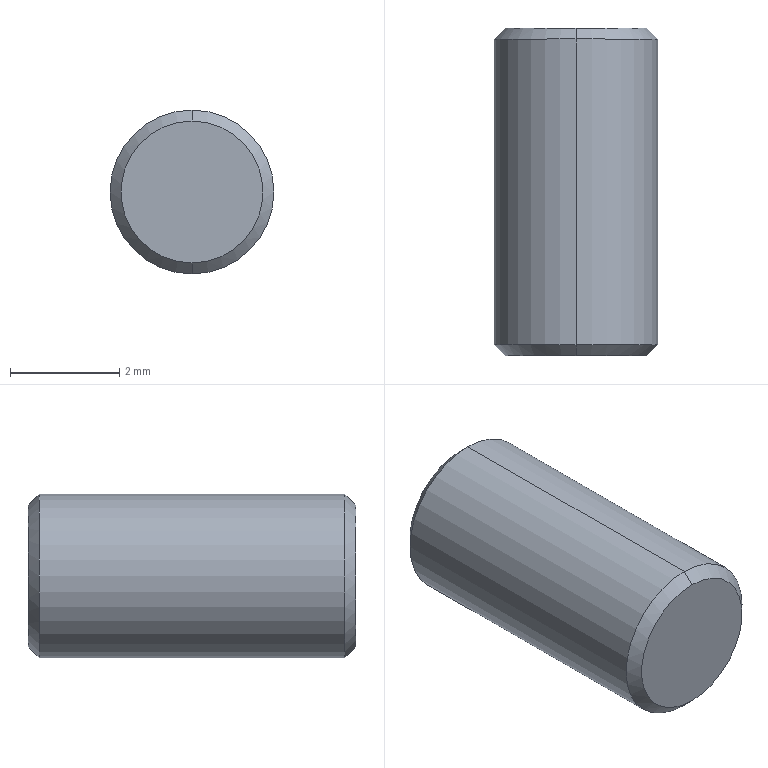Part | SolidWorks | features Chamfer 1, Extrusion 1 | 1 solid | 8 faces | box 3 x 6 x 3 mm | volume 42.051 mm3 | cone 4 | cylinder 2 | plane 2 | commonest cylinder face diameters 3 x2
STEP:
#1=CARTESIAN_POINT('',(0.,6.,1.3));
#2=VERTEX_POINT('',#1);
#3=CARTESIAN_POINT('',(0.,6.,-1.3));
#4=VERTEX_POINT('',#3);
#5=CARTESIAN_POINT('',(0.,6.,0.));
#6=DIRECTION('',(0.,1.,0.));
#7=DIRECTION('',(0.,0.,1.));
#8=AXIS2_PLACEMENT_3D('',#5,#6,#7);
#9=CIRCLE('',#8,1.3);
#10=EDGE_CURVE('',#2,#4,#9,.T.);
#11=ORIENTED_EDGE('',*,*,#10,.F.);
#12=CARTESIAN_POINT('',(0.,5.8,1.5));
#13=VERTEX_POINT('',#12);
#14=CARTESIAN_POINT('',(0.,6.,1.3));
#15=DIRECTION('',(0.,-0.7071,0.7071));
#16=VECTOR('',#15,1000.);
#17=LINE('',#14,#16);
#18=EDGE_CURVE('',#2,#13,#17,.T.);
#19=ORIENTED_EDGE('',*,*,#18,.T.);
#20=CARTESIAN_POINT('',(0.,5.8,-1.5));
#21=VERTEX_POINT('',#20);
#22=CARTESIAN_POINT('',(0.,5.8,0.));
#23=DIRECTION('',(0.,-1.,0.));
#24=DIRECTION('',(0.,0.,1.));
#25=AXIS2_PLACEMENT_3D('',#22,#23,#24);
#26=CIRCLE('',#25,1.5);
#27=EDGE_CURVE('',#21,#13,#26,.T.);
#28=ORIENTED_EDGE('',*,*,#27,.F.);
#29=CARTESIAN_POINT('',(0.,6.,-1.3));
#30=DIRECTION('',(0.,-0.7071,-0.7071));
#31=VECTOR('',#30,1000.);
#32=LINE('',#29,#31);
#33=EDGE_CURVE('',#4,#21,#32,.T.);
#34=ORIENTED_EDGE('',*,*,#33,.F.);
#35=EDGE_LOOP('',(#11,#19,#28,#34));
#36=FACE_OUTER_BOUND('',#35,.T.);
#37=CARTESIAN_POINT('',(0.,6.,0.));
#38=DIRECTION('',(0.,-1.,0.));
#39=DIRECTION('',(0.,0.,-1.));
#40=AXIS2_PLACEMENT_3D('',#37,#38,#39);
#41=CONICAL_SURFACE('',#40,1.3,0.7854);
#42=ADVANCED_FACE('',(#36),#41,.T.);
#43=CARTESIAN_POINT('',(0.,0.,-1.3));
#44=VERTEX_POINT('',#43);
#45=CARTESIAN_POINT('',(0.,0.,1.3));
#46=VERTEX_POINT('',#45);
#47=CARTESIAN_POINT('',(0.,0.,0.));
#48=DIRECTION('',(0.,-1.,0.));
#49=DIRECTION('',(0.,0.,1.));
#50=AXIS2_PLACEMENT_3D('',#47,#48,#49);
#51=CIRCLE('',#50,1.3);
#52=EDGE_CURVE('',#44,#46,#51,.T.);
#53=ORIENTED_EDGE('',*,*,#52,.F.);
#54=CARTESIAN_POINT('',(0.,0.2,-1.5));
#55=VERTEX_POINT('',#54);
#56=CARTESIAN_POINT('',(0.,0.2,-1.5));
#57=DIRECTION('',(0.,0.7071,-0.7071));
#58=VECTOR('',#57,1000.);
#59=LINE('',#56,#58);
#60=EDGE_CURVE('',#44,#55,#59,.T.);
#61=ORIENTED_EDGE('',*,*,#60,.T.);
#62=CARTESIAN_POINT('',(0.,0.2,1.5));
#63=VERTEX_POINT('',#62);
#64=CARTESIAN_POINT('',(0.,0.2,0.));
#65=DIRECTION('',(0.,1.,0.));
#66=DIRECTION('',(0.,0.,1.));
#67=AXIS2_PLACEMENT_3D('',#64,#65,#66);
#68=CIRCLE('',#67,1.5);
#69=EDGE_CURVE('',#63,#55,#68,.T.);
#70=ORIENTED_EDGE('',*,*,#69,.F.);
#71=CARTESIAN_POINT('',(0.,0.2,1.5));
#72=DIRECTION('',(0.,0.7071,0.7071));
#73=VECTOR('',#72,1000.);
#74=LINE('',#71,#73);
#75=EDGE_CURVE('',#46,#63,#74,.T.);
#76=ORIENTED_EDGE('',*,*,#75,.F.);
#77=EDGE_LOOP('',(#53,#61,#70,#76));
#78=FACE_OUTER_BOUND('',#77,.T.);
#79=CARTESIAN_POINT('',(0.,0.2,0.));
#80=DIRECTION('',(0.,1.,0.));
#81=DIRECTION('',(0.,0.,1.));
#82=AXIS2_PLACEMENT_3D('',#79,#80,#81);
#83=CONICAL_SURFACE('',#82,1.5,0.7854);
#84=ADVANCED_FACE('',(#78),#83,.T.);
#85=ORIENTED_EDGE('',*,*,#27,.T.);
#86=CARTESIAN_POINT('',(0.,6.,1.5));
#87=DIRECTION('',(0.,-1.,0.));
#88=VECTOR('',#87,1000.);
#89=LINE('',#86,#88);
#90=EDGE_CURVE('',#13,#63,#89,.T.);
#91=ORIENTED_EDGE('',*,*,#90,.T.);
#92=ORIENTED_EDGE('',*,*,#69,.T.);
#93=CARTESIAN_POINT('',(0.,6.,-1.5));
#94=DIRECTION('',(0.,-1.,0.));
#95=VECTOR('',#94,1000.);
#96=LINE('',#93,#95);
#97=EDGE_CURVE('',#21,#55,#96,.T.);
#98=ORIENTED_EDGE('',*,*,#97,.F.);
#99=EDGE_LOOP('',(#85,#91,#92,#98));
#100=FACE_OUTER_BOUND('',#99,.T.);
#101=CARTESIAN_POINT('',(0.,6.,0.));
#102=DIRECTION('',(0.,-1.,0.));
#103=DIRECTION('',(0.,0.,-1.));
#104=AXIS2_PLACEMENT_3D('',#101,#102,#103);
#105=CYLINDRICAL_SURFACE('',#104,1.5);
#106=ADVANCED_FACE('',(#100),#105,.T.);
#107=ORIENTED_EDGE('',*,*,#90,.F.);
#108=CARTESIAN_POINT('',(0.,5.8,0.));
#109=DIRECTION('',(0.,-1.,0.));
#110=DIRECTION('',(0.,0.,1.));
#111=AXIS2_PLACEMENT_3D('',#108,#109,#110);
#112=CIRCLE('',#111,1.5);
#113=EDGE_CURVE('',#13,#21,#112,.T.);
#114=ORIENTED_EDGE('',*,*,#113,.T.);
#115=ORIENTED_EDGE('',*,*,#97,.T.);
#116=CARTESIAN_POINT('',(0.,0.2,0.));
#117=DIRECTION('',(0.,1.,0.));
#118=DIRECTION('',(0.,0.,1.));
#119=AXIS2_PLACEMENT_3D('',#116,#117,#118);
#120=CIRCLE('',#119,1.5);
#121=EDGE_CURVE('',#55,#63,#120,.T.);
#122=ORIENTED_EDGE('',*,*,#121,.T.);
#123=EDGE_LOOP('',(#107,#114,#115,#122));
#124=FACE_OUTER_BOUND('',#123,.T.);
#125=CARTESIAN_POINT('',(0.,6.,0.));
#126=DIRECTION('',(0.,-1.,0.));
#127=DIRECTION('',(0.,0.,-1.));
#128=AXIS2_PLACEMENT_3D('',#125,#126,#127);
#129=CYLINDRICAL_SURFACE('',#128,1.5);
#130=ADVANCED_FACE('',(#124),#129,.T.);
#131=CARTESIAN_POINT('',(0.,6.,0.));
#132=DIRECTION('',(0.,1.,0.));
#133=DIRECTION('',(0.,0.,1.));
#134=AXIS2_PLACEMENT_3D('',#131,#132,#133);
#135=CIRCLE('',#134,1.3);
#136=EDGE_CURVE('',#4,#2,#135,.T.);
#137=ORIENTED_EDGE('',*,*,#136,.T.);
#138=ORIENTED_EDGE('',*,*,#10,.T.);
#139=EDGE_LOOP('',(#137,#138));
#140=FACE_OUTER_BOUND('',#139,.T.);
#141=CARTESIAN_POINT('',(0.,6.,0.));
#142=DIRECTION('',(0.,1.,0.));
#143=DIRECTION('',(0.,0.,1.));
#144=AXIS2_PLACEMENT_3D('',#141,#142,#143);
#145=PLANE('',#144);
#146=ADVANCED_FACE('',(#140),#145,.T.);
#147=CARTESIAN_POINT('',(0.,0.,0.));
#148=DIRECTION('',(0.,-1.,0.));
#149=DIRECTION('',(0.,0.,1.));
#150=AXIS2_PLACEMENT_3D('',#147,#148,#149);
#151=CIRCLE('',#150,1.3);
#152=EDGE_CURVE('',#46,#44,#151,.T.);
#153=ORIENTED_EDGE('',*,*,#152,.T.);
#154=ORIENTED_EDGE('',*,*,#52,.T.);
#155=EDGE_LOOP('',(#153,#154));
#156=FACE_OUTER_BOUND('',#155,.T.);
#157=CARTESIAN_POINT('',(0.,0.,0.));
#158=DIRECTION('',(0.,1.,0.));
#159=DIRECTION('',(0.,0.,1.));
#160=AXIS2_PLACEMENT_3D('',#157,#158,#159);
#161=PLANE('',#160);
#162=ADVANCED_FACE('',(#156),#161,.F.);
#163=ORIENTED_EDGE('',*,*,#60,.F.);
#164=ORIENTED_EDGE('',*,*,#152,.F.);
#165=ORIENTED_EDGE('',*,*,#75,.T.);
#166=ORIENTED_EDGE('',*,*,#121,.F.);
#167=EDGE_LOOP('',(#163,#164,#165,#166));
#168=FACE_OUTER_BOUND('',#167,.T.);
#169=CARTESIAN_POINT('',(0.,0.2,0.));
#170=DIRECTION('',(0.,1.,0.));
#171=DIRECTION('',(0.,0.,1.));
#172=AXIS2_PLACEMENT_3D('',#169,#170,#171);
#173=CONICAL_SURFACE('',#172,1.5,0.7854);
#174=ADVANCED_FACE('',(#168),#173,.T.);
#175=ORIENTED_EDGE('',*,*,#18,.F.);
#176=ORIENTED_EDGE('',*,*,#136,.F.);
#177=ORIENTED_EDGE('',*,*,#33,.T.);
#178=ORIENTED_EDGE('',*,*,#113,.F.);
#179=EDGE_LOOP('',(#175,#176,#177,#178));
#180=FACE_OUTER_BOUND('',#179,.T.);
#181=CARTESIAN_POINT('',(0.,6.,0.));
#182=DIRECTION('',(0.,-1.,0.));
#183=DIRECTION('',(0.,0.,-1.));
#184=AXIS2_PLACEMENT_3D('',#181,#182,#183);
#185=CONICAL_SURFACE('',#184,1.3,0.7854);
#186=ADVANCED_FACE('',(#180),#185,.T.);
#187=CLOSED_SHELL('',(#42,#84,#106,#130,#146,#162,#174,#186));
#188=MANIFOLD_SOLID_BREP('',#187);
#189=CARTESIAN_POINT('',(0.,0.,0.));
#190=DIRECTION('',(0.,0.,1.));
#191=DIRECTION('',(1.,0.,0.));
#192=AXIS2_PLACEMENT_3D('',#189,#190,#191);
#193=(LENGTH_UNIT()NAMED_UNIT(*)SI_UNIT(.MILLI.,.METRE.));
#194=UNCERTAINTY_MEASURE_WITH_UNIT(LENGTH_MEASURE(0.00001),#193,'','');
#195=(NAMED_UNIT(*)PLANE_ANGLE_UNIT()SI_UNIT($,.RADIAN.));
#196=(NAMED_UNIT(*)SI_UNIT($,.STERADIAN.)SOLID_ANGLE_UNIT());
#197=(GEOMETRIC_REPRESENTATION_CONTEXT(3)GLOBAL_UNCERTAINTY_ASSIGNED_CONTEXT((#194))GLOBAL_UNIT_ASSIGNED_CONTEXT((#193,#195,#196))REPRESENTATION_CONTEXT('',''));
#198=ADVANCED_BREP_SHAPE_REPRESENTATION('',(#188,#192),#197);